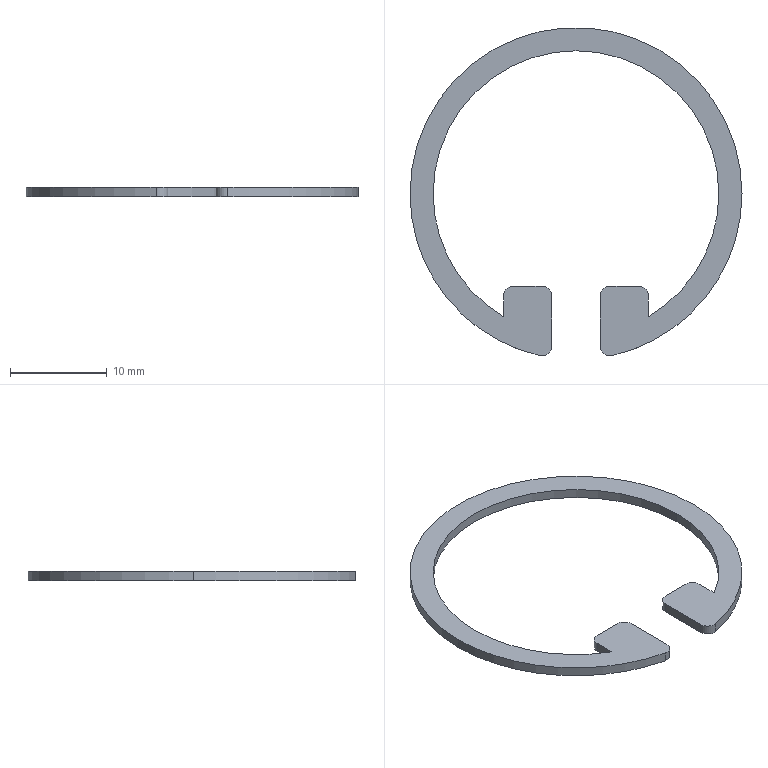Part | STEP file | Inner clip | 1 solid | 20 faces | box 34.4 x 34.017 x 1 mm | volume 270.275 mm3 | cylinder 12 | plane 8 | commonest cylinder face diameters 2 x6 29.6 x3 34.4 x3